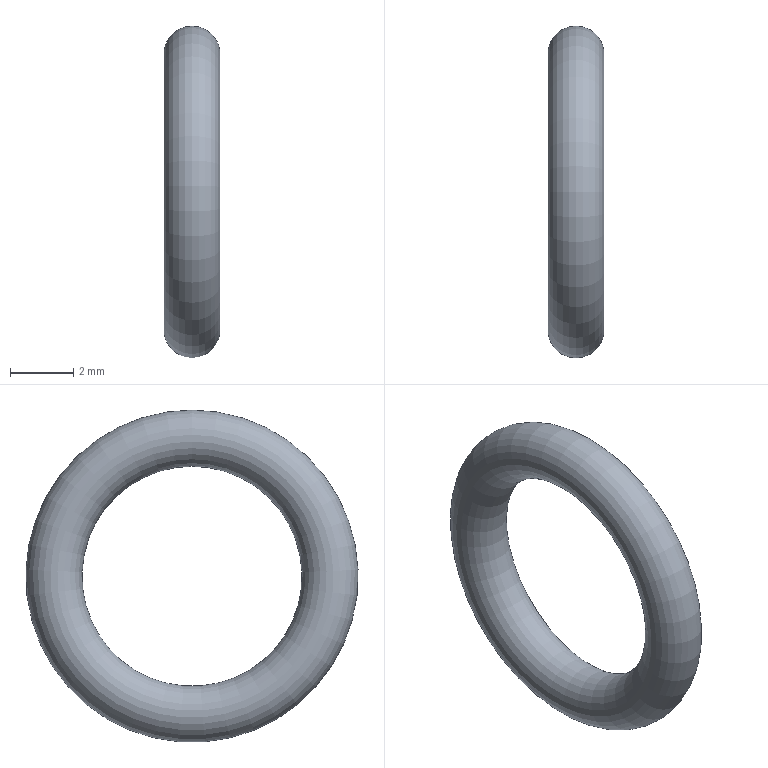Part | NX | features solid 2 | 1 solid | 1 faces | box 1.778 x 10.516 x 10.516 mm | volume 68.155 mm3 | torus 1
STEP:
#1=CARTESIAN_POINT('',(4.702,0.,3.48));
#2=VERTEX_POINT('',#1);
#3=VERTEX_LOOP('',#2);
#4=FACE_BOUND('',#3,.T.);
#5=CARTESIAN_POINT('',(4.702,0.,0.));
#6=DIRECTION('',(-1.,0.,0.));
#7=DIRECTION('',(0.,0.,1.));
#8=AXIS2_PLACEMENT_3D('',#5,#6,#7);
#9=TOROIDAL_SURFACE('',#8,4.369,0.889);
#10=ADVANCED_FACE('',(#4),#9,.T.);
#11=CLOSED_SHELL('',(#10));
#12=MANIFOLD_SOLID_BREP('',#11);
#13=(LENGTH_UNIT()NAMED_UNIT(*)SI_UNIT(.MILLI.,.METRE.));
#14=UNCERTAINTY_MEASURE_WITH_UNIT(LENGTH_MEASURE(0.00001),#13,'','');
#15=(NAMED_UNIT(*)PLANE_ANGLE_UNIT()SI_UNIT($,.RADIAN.));
#16=(NAMED_UNIT(*)SI_UNIT($,.STERADIAN.)SOLID_ANGLE_UNIT());
#17=(GEOMETRIC_REPRESENTATION_CONTEXT(3)GLOBAL_UNCERTAINTY_ASSIGNED_CONTEXT((#14))GLOBAL_UNIT_ASSIGNED_CONTEXT((#13,#15,#16))REPRESENTATION_CONTEXT('',''));
#18=ADVANCED_BREP_SHAPE_REPRESENTATION('',(#12),#17);